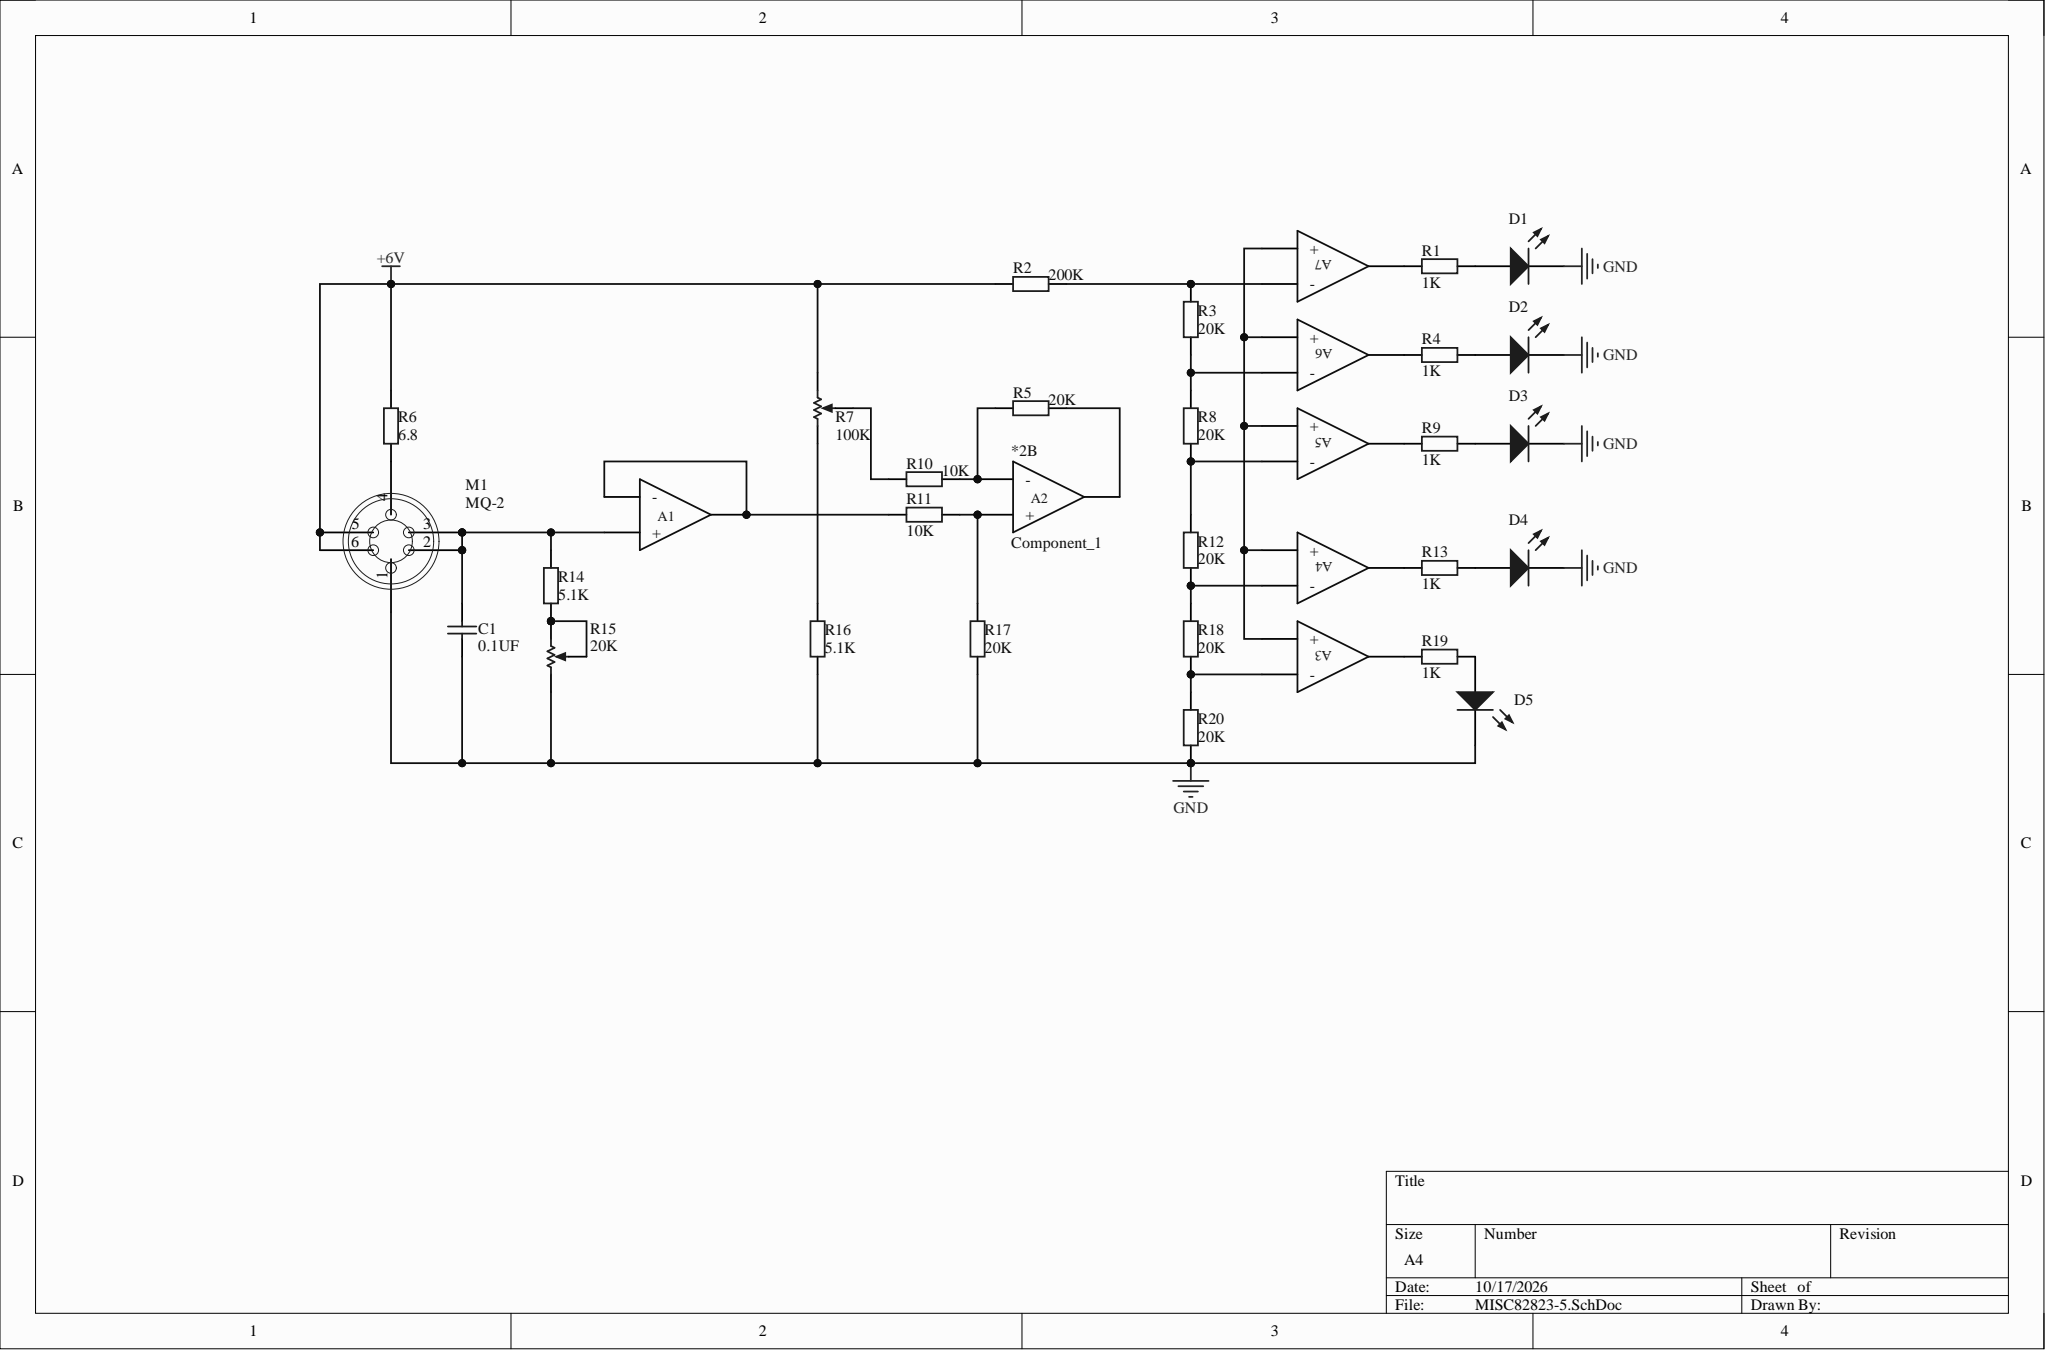Circuit board | Altium Designer | 29 parts | 27 nets
Bill of materials:
Comment,Description,Designator,Footprint,LibRef,Quantity
"Component_2","","*1","DIP14","Component_2","1"
"Component_1","","*2","DIP14","Component_1","1"
"0.1UF","Capacitor","C1","RAD-0.1","Cap","1"
"LED3","Typical BLUE SiC LED","D1, D2, D3, D4, D5","LED3MM","LED3","5"
"MQ-2","Gas sensor","M1","MQ-2","MQ-2","1"
"1K","Resistor","R1, R4, R9, R13, R19","AXIAL-0.4","Res2","5"
"200K","Resistor","R2","AXIAL-0.4","Res2","1"
"20K","Resistor","R3, R5, R8, R12, R17, R18, R20","AXIAL-0.4","Res2","7"
"6.8","Resistor","R6","AXIAL-0.4","Res2","1"
"100K","Potentiometer","R7","VR5","RPot","1"
"10K","Resistor","R10, R11","AXIAL-0.4","Res2","2"
"5.1K","Resistor","R14, R16","AXIAL-0.4","Res2","2"
"20K","Potentiometer","R15","VR5","RPot","1"
Netlist (Protel format):
[
*1
DIP14
Component_2



]
[
*2
DIP14
Component_1



]
[
C1
RAD-0.1
0.1UF



]
[
D1
LED3MM
LED3



]
[
D2
LED3MM
LED3



]
[
D3
LED3MM
LED3



]
[
D4
LED3MM
LED3



]
[
D5
LED3MM
LED3



]
[
M1
MQ-2
MQ-2



]
[
R1
AXIAL-0.4
1K



]
[
R2
AXIAL-0.4
200K



]
[
R3
AXIAL-0.4
20K



]
[
R4
AXIAL-0.4
1K



]
[
R5
AXIAL-0.4
20K



]
[
R6
AXIAL-0.4
6.8



]
[
R7
VR5
100K



]
[
R8
AXIAL-0.4
20K



]
[
R9
AXIAL-0.4
1K



]
[
R10
AXIAL-0.4
10K



]
[
R11
AXIAL-0.4
10K



]
[
R12
AXIAL-0.4
20K



]
[
R13
AXIAL-0.4
1K



]
[
R14
AXIAL-0.4
5.1K



]
[
R15
VR5
20K



]
[
R16
AXIAL-0.4
5.1K



]
[
R17
AXIAL-0.4
20K



]
[
R18
AXIAL-0.4
20K



]
[
R19
AXIAL-0.4
1K



]
[
R20
AXIAL-0.4
20K



]
(
NetR14_1
R14-1
R15-2
R15-3
)
(
NetR7_3
R7-3
R10-2
)
(
NetR7_1
R7-1
R16-2
)
(
NetM1_4
M1-4
R6-1
)
(
NetD5_1
D5-1
R19-2
)
(
NetD4_1
D4-1
R13-2
)
(
NetD3_1
D3-1
R9-2
)
(
NetD2_1
D2-1
R4-2
)
(
NetD1_1
D1-1
R1-2
)
(
Net*2_10
*2-10
R19-1
)
(
Net*2_8
*2-8
R18-2
R20-1
)
(
Net*2_7
*2-7
R5-1
)
(
Net*2_6
*2-6
R11-1
R17-2
)
(
Net*2_5
*2-5
R5-2
R10-1
)
(
Net*2_3
*2-3
C1-2
M1-2
M1-3
R14-2
)
(
Net*2_2
*2-2
*2-4
R11-2
)
(
Net*1_13
*1-13
R1-1
)
(
Net*1_11
*1-11
R2-1
R3-1
)
(
Net*1_10
*1-10
R4-1
)
(
Net*1_8
*1-8
R3-2
R8-1
)
(
Net*1_7
*1-7
R9-1
)
(
Net*1_5
*1-5
R8-2
R12-1
)
(
Net*1_4
*1-4
R13-1
)
(
Net*1_3
*1-3
*1-6
*1-9
*1-12
*2-9
)
(
Net*1_2
*1-2
R12-2
R18-1
)
(
GND
C1-1
D1-2
D2-2
D3-2
D4-2
D5-2
M1-1
R15-1
R16-1
R17-1
R20-2
)
(
+6V
M1-5
M1-6
R2-2
R6-2
R7-2
)